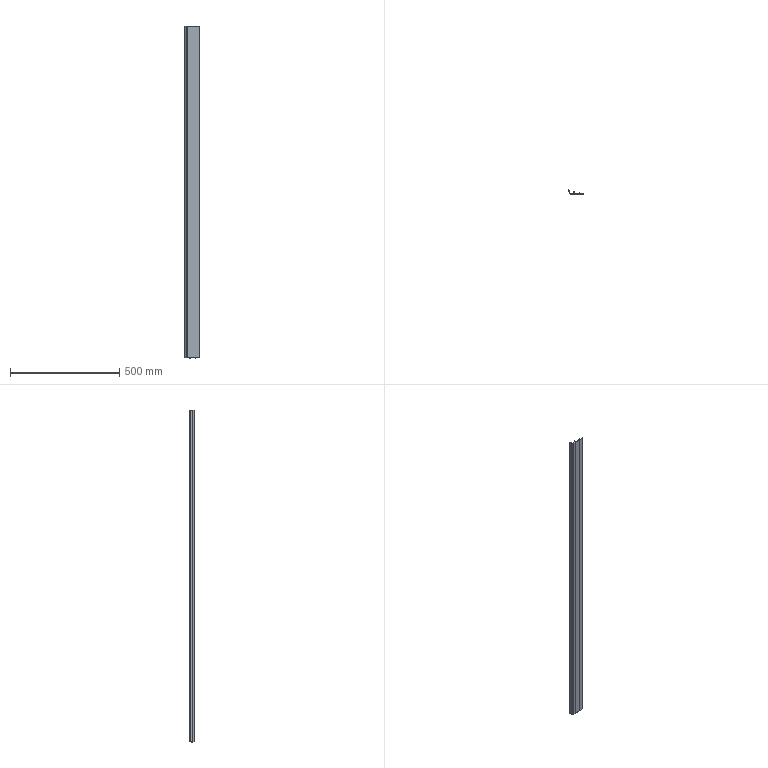Part | STEP file | 51E-01200JG10 | 1 solid | 49 faces | box 67.801 x 18.48 x 1520 mm | volume 173727 mm3 | cylinder 28 | plane 21 | commonest cylinder face diameters 0.4 x11 0.6 x3 1 x3 1.2 x2 1.4 x2 4 x2